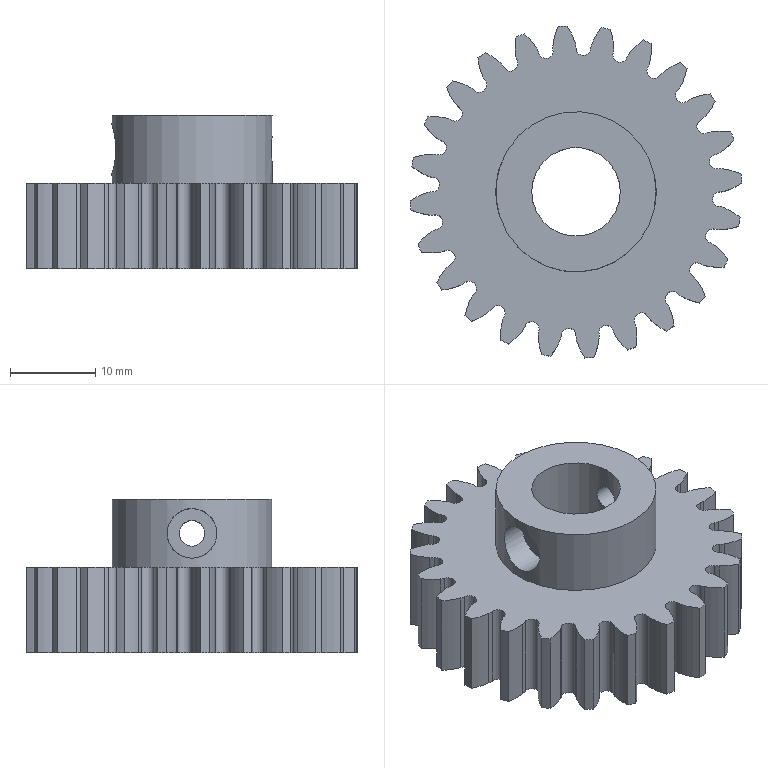Part | NX | features BREP 2, DATUM_CSYS 1, UNITE 1 | 1 solid | 155 faces | box 38.944 x 38.944 x 18 mm | volume 9823 mm3 | cylinder 150 | plane 5 | commonest cylinder face diameters 4 x48 14.148 x48 1.7 x24 39 x24 3 x2 5.82 x1